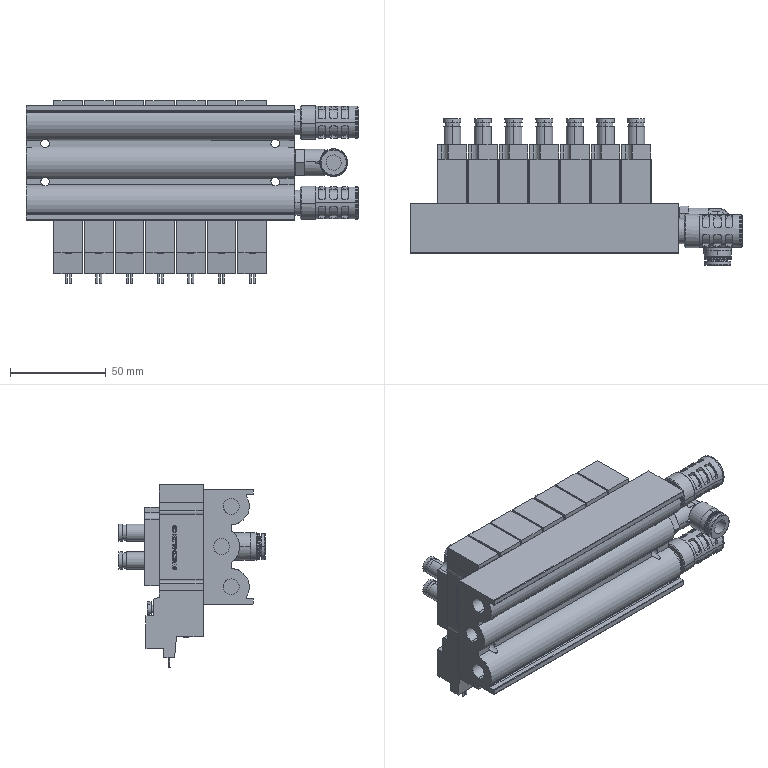Part | NX | 11 solids | 4820 faces | volume 403957 mm3 | plane 4148 | cylinder 556 | cone 109 | torus 4 | sphere 2 | spline 1 | commonest cylinder face diameters 2 x96 4 x84 9 x56 2.5 x42 7.938 x42 1 x30